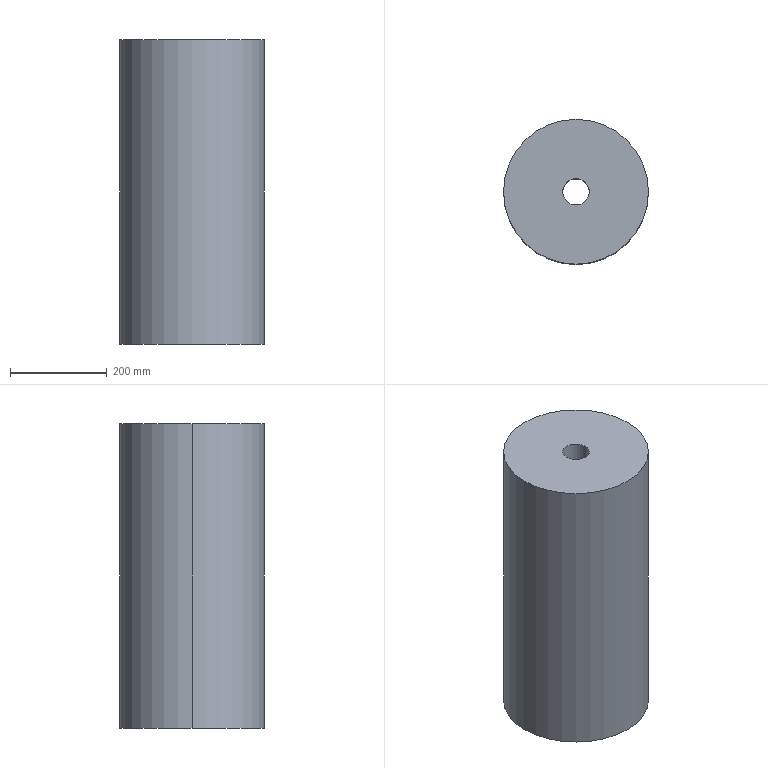Part | STEP file | Coil stock | 1 solid | 6 faces | box 300 x 300 x 630 mm | volume 43035303 mm3 | cylinder 4 | plane 2 | commonest cylinder face diameters 55 x2 300 x2
STEP:
#1=CARTESIAN_POINT('',(0.,0.,0.));
#2=DIRECTION('',(0.,0.,1.));
#3=DIRECTION('',(1.,0.,0.));
#4=AXIS2_PLACEMENT_3D('',#1,#2,#3);
#5=CARTESIAN_POINT('',(150.,0.,0.));
#6=VERTEX_POINT('',#5);
#7=CARTESIAN_POINT('',(-150.,0.,0.));
#8=VERTEX_POINT('',#7);
#9=CARTESIAN_POINT('',(0.,0.,0.));
#10=DIRECTION('',(0.,0.,1.));
#11=DIRECTION('',(1.,0.,0.));
#12=AXIS2_PLACEMENT_3D('',#9,#10,#11);
#13=CIRCLE('',#12,150.);
#14=CARTESIAN_POINT('',(0.,0.,0.));
#15=DIRECTION('',(0.,0.,1.));
#16=DIRECTION('',(1.,0.,0.));
#17=AXIS2_PLACEMENT_3D('',#14,#15,#16);
#18=CYLINDRICAL_SURFACE('',#17,150.);
#19=CARTESIAN_POINT('',(0.,0.));
#20=DIRECTION('',(1.,0.));
#21=VECTOR('',#20,1.);
#22=LINE('',#19,#21);
#23=(GEOMETRIC_REPRESENTATION_CONTEXT(2)PARAMETRIC_REPRESENTATION_CONTEXT()REPRESENTATION_CONTEXT('',''));
#24=DEFINITIONAL_REPRESENTATION('',(#22),#23);
#25=PCURVE('',#18,#24);
#26=CARTESIAN_POINT('',(0.,0.,0.));
#27=DIRECTION('',(0.,0.,-1.));
#28=DIRECTION('',(-1.,0.,0.));
#29=AXIS2_PLACEMENT_3D('',#26,#27,#28);
#30=PLANE('',#29);
#31=CARTESIAN_POINT('',(-150.,0.));
#32=CARTESIAN_POINT('',(-150.,259.808));
#33=CARTESIAN_POINT('',(75.,129.904));
#34=CARTESIAN_POINT('',(300.,0.));
#35=CARTESIAN_POINT('',(75.,-129.904));
#36=CARTESIAN_POINT('',(-150.,-259.808));
#37=CARTESIAN_POINT('',(-150.,0.));
#38=(BOUNDED_CURVE()B_SPLINE_CURVE(2,(#31,#32,#33,#34,#35,#36,#37),.UNSPECIFIED.,.T.,.F.)B_SPLINE_CURVE_WITH_KNOTS((1,2,2,2,2,1),(-2.094,0.,2.094,4.189,6.283,8.378),.UNSPECIFIED.)CURVE()GEOMETRIC_REPRESENTATION_ITEM()RATIONAL_B_SPLINE_CURVE((1.,0.5,1.,0.5,1.,0.5,1.))REPRESENTATION_ITEM(''));
#39=(GEOMETRIC_REPRESENTATION_CONTEXT(2)PARAMETRIC_REPRESENTATION_CONTEXT()REPRESENTATION_CONTEXT('',''));
#40=DEFINITIONAL_REPRESENTATION('',(#38),#39);
#41=PCURVE('',#30,#40);
#42=SURFACE_CURVE('',#13,(#25,#41),.PCURVE_S1.);
#43=EDGE_CURVE('',#6,#8,#42,.T.);
#44=ORIENTED_EDGE('',*,*,#43,.T.);
#45=CARTESIAN_POINT('',(-150.,0.,630.));
#46=VERTEX_POINT('',#45);
#47=CARTESIAN_POINT('',(-150.,0.,0.));
#48=DIRECTION('',(0.,0.,1.));
#49=VECTOR('',#48,1.);
#50=LINE('',#47,#49);
#51=CARTESIAN_POINT('',(3.142,0.));
#52=DIRECTION('',(0.,1.));
#53=VECTOR('',#52,1.);
#54=LINE('',#51,#53);
#55=(GEOMETRIC_REPRESENTATION_CONTEXT(2)PARAMETRIC_REPRESENTATION_CONTEXT()REPRESENTATION_CONTEXT('',''));
#56=DEFINITIONAL_REPRESENTATION('',(#54),#55);
#57=PCURVE('',#18,#56);
#58=CARTESIAN_POINT('',(0.,0.,0.));
#59=DIRECTION('',(0.,0.,1.));
#60=DIRECTION('',(1.,0.,0.));
#61=AXIS2_PLACEMENT_3D('',#58,#59,#60);
#62=CYLINDRICAL_SURFACE('',#61,150.);
#63=CARTESIAN_POINT('',(3.142,0.));
#64=DIRECTION('',(0.,1.));
#65=VECTOR('',#64,1.);
#66=LINE('',#63,#65);
#67=(GEOMETRIC_REPRESENTATION_CONTEXT(2)PARAMETRIC_REPRESENTATION_CONTEXT()REPRESENTATION_CONTEXT('',''));
#68=DEFINITIONAL_REPRESENTATION('',(#66),#67);
#69=PCURVE('',#62,#68);
#70=SURFACE_CURVE('',#50,(#57,#69),.PCURVE_S1.);
#71=EDGE_CURVE('',#8,#46,#70,.T.);
#72=ORIENTED_EDGE('',*,*,#71,.T.);
#73=CARTESIAN_POINT('',(150.,0.,630.));
#74=VERTEX_POINT('',#73);
#75=CARTESIAN_POINT('',(0.,0.,630.));
#76=DIRECTION('',(0.,0.,-1.));
#77=DIRECTION('',(1.,0.,0.));
#78=AXIS2_PLACEMENT_3D('',#75,#76,#77);
#79=CIRCLE('',#78,150.);
#80=CARTESIAN_POINT('',(6.283,630.));
#81=DIRECTION('',(-1.,0.));
#82=VECTOR('',#81,1.);
#83=LINE('',#80,#82);
#84=(GEOMETRIC_REPRESENTATION_CONTEXT(2)PARAMETRIC_REPRESENTATION_CONTEXT()REPRESENTATION_CONTEXT('',''));
#85=DEFINITIONAL_REPRESENTATION('',(#83),#84);
#86=PCURVE('',#18,#85);
#87=CARTESIAN_POINT('',(0.,0.,630.));
#88=DIRECTION('',(0.,0.,-1.));
#89=DIRECTION('',(-1.,0.,0.));
#90=AXIS2_PLACEMENT_3D('',#87,#88,#89);
#91=PLANE('',#90);
#92=CARTESIAN_POINT('',(0.,0.));
#93=DIRECTION('',(-1.,0.));
#94=AXIS2_PLACEMENT_2D('',#92,#93);
#95=CIRCLE('',#94,150.);
#96=(GEOMETRIC_REPRESENTATION_CONTEXT(2)PARAMETRIC_REPRESENTATION_CONTEXT()REPRESENTATION_CONTEXT('',''));
#97=DEFINITIONAL_REPRESENTATION('',(#95),#96);
#98=PCURVE('',#91,#97);
#99=SURFACE_CURVE('',#79,(#86,#98),.PCURVE_S1.);
#100=EDGE_CURVE('',#46,#74,#99,.T.);
#101=ORIENTED_EDGE('',*,*,#100,.T.);
#102=CARTESIAN_POINT('',(150.,0.,0.));
#103=DIRECTION('',(0.,0.,1.));
#104=VECTOR('',#103,1.);
#105=LINE('',#102,#104);
#106=CARTESIAN_POINT('',(0.,0.));
#107=DIRECTION('',(0.,1.));
#108=VECTOR('',#107,1.);
#109=LINE('',#106,#108);
#110=(GEOMETRIC_REPRESENTATION_CONTEXT(2)PARAMETRIC_REPRESENTATION_CONTEXT()REPRESENTATION_CONTEXT('',''));
#111=DEFINITIONAL_REPRESENTATION('',(#109),#110);
#112=PCURVE('',#18,#111);
#113=CARTESIAN_POINT('',(6.283,0.));
#114=DIRECTION('',(0.,1.));
#115=VECTOR('',#114,1.);
#116=LINE('',#113,#115);
#117=(GEOMETRIC_REPRESENTATION_CONTEXT(2)PARAMETRIC_REPRESENTATION_CONTEXT()REPRESENTATION_CONTEXT('',''));
#118=DEFINITIONAL_REPRESENTATION('',(#116),#117);
#119=PCURVE('',#62,#118);
#120=SURFACE_CURVE('',#105,(#112,#119),.PCURVE_S1.);
#121=EDGE_CURVE('',#6,#74,#120,.T.);
#122=ORIENTED_EDGE('',*,*,#121,.F.);
#123=EDGE_LOOP('',(#44,#72,#101,#122));
#124=FACE_BOUND('',#123,.T.);
#125=ADVANCED_FACE('',(#124),#18,.T.);
#126=CARTESIAN_POINT('',(27.5,0.,0.));
#127=VERTEX_POINT('',#126);
#128=CARTESIAN_POINT('',(27.5,0.,630.));
#129=VERTEX_POINT('',#128);
#130=CARTESIAN_POINT('',(27.5,0.,0.));
#131=DIRECTION('',(0.,0.,1.));
#132=VECTOR('',#131,1.);
#133=LINE('',#130,#132);
#134=CARTESIAN_POINT('',(0.,0.,0.));
#135=DIRECTION('',(0.,0.,1.));
#136=DIRECTION('',(1.,0.,0.));
#137=AXIS2_PLACEMENT_3D('',#134,#135,#136);
#138=CYLINDRICAL_SURFACE('',#137,27.5);
#139=CARTESIAN_POINT('',(6.283,0.));
#140=DIRECTION('',(0.,1.));
#141=VECTOR('',#140,1.);
#142=LINE('',#139,#141);
#143=(GEOMETRIC_REPRESENTATION_CONTEXT(2)PARAMETRIC_REPRESENTATION_CONTEXT()REPRESENTATION_CONTEXT('',''));
#144=DEFINITIONAL_REPRESENTATION('',(#142),#143);
#145=PCURVE('',#138,#144);
#146=CARTESIAN_POINT('',(0.,0.,0.));
#147=DIRECTION('',(0.,0.,1.));
#148=DIRECTION('',(1.,0.,0.));
#149=AXIS2_PLACEMENT_3D('',#146,#147,#148);
#150=CYLINDRICAL_SURFACE('',#149,27.5);
#151=CARTESIAN_POINT('',(0.,0.));
#152=DIRECTION('',(0.,1.));
#153=VECTOR('',#152,1.);
#154=LINE('',#151,#153);
#155=(GEOMETRIC_REPRESENTATION_CONTEXT(2)PARAMETRIC_REPRESENTATION_CONTEXT()REPRESENTATION_CONTEXT('',''));
#156=DEFINITIONAL_REPRESENTATION('',(#154),#155);
#157=PCURVE('',#150,#156);
#158=SURFACE_CURVE('',#133,(#145,#157),.PCURVE_S1.);
#159=EDGE_CURVE('',#127,#129,#158,.T.);
#160=ORIENTED_EDGE('',*,*,#159,.T.);
#161=CARTESIAN_POINT('',(-27.5,0.,630.));
#162=VERTEX_POINT('',#161);
#163=CARTESIAN_POINT('',(0.,0.,630.));
#164=DIRECTION('',(0.,0.,1.));
#165=DIRECTION('',(1.,0.,0.));
#166=AXIS2_PLACEMENT_3D('',#163,#164,#165);
#167=CIRCLE('',#166,27.5);
#168=CARTESIAN_POINT('',(0.,630.));
#169=DIRECTION('',(1.,0.));
#170=VECTOR('',#169,1.);
#171=LINE('',#168,#170);
#172=(GEOMETRIC_REPRESENTATION_CONTEXT(2)PARAMETRIC_REPRESENTATION_CONTEXT()REPRESENTATION_CONTEXT('',''));
#173=DEFINITIONAL_REPRESENTATION('',(#171),#172);
#174=PCURVE('',#138,#173);
#175=CARTESIAN_POINT('',(-27.5,0.));
#176=CARTESIAN_POINT('',(-27.5,47.631));
#177=CARTESIAN_POINT('',(13.75,23.816));
#178=CARTESIAN_POINT('',(55.,0.));
#179=CARTESIAN_POINT('',(13.75,-23.816));
#180=CARTESIAN_POINT('',(-27.5,-47.631));
#181=CARTESIAN_POINT('',(-27.5,0.));
#182=(BOUNDED_CURVE()B_SPLINE_CURVE(2,(#175,#176,#177,#178,#179,#180,#181),.UNSPECIFIED.,.T.,.F.)B_SPLINE_CURVE_WITH_KNOTS((1,2,2,2,2,1),(-2.094,0.,2.094,4.189,6.283,8.378),.UNSPECIFIED.)CURVE()GEOMETRIC_REPRESENTATION_ITEM()RATIONAL_B_SPLINE_CURVE((1.,0.5,1.,0.5,1.,0.5,1.))REPRESENTATION_ITEM(''));
#183=(GEOMETRIC_REPRESENTATION_CONTEXT(2)PARAMETRIC_REPRESENTATION_CONTEXT()REPRESENTATION_CONTEXT('',''));
#184=DEFINITIONAL_REPRESENTATION('',(#182),#183);
#185=PCURVE('',#91,#184);
#186=SURFACE_CURVE('',#167,(#174,#185),.PCURVE_S1.);
#187=EDGE_CURVE('',#162,#129,#186,.T.);
#188=ORIENTED_EDGE('',*,*,#187,.F.);
#189=CARTESIAN_POINT('',(-27.5,0.,0.));
#190=VERTEX_POINT('',#189);
#191=CARTESIAN_POINT('',(-27.5,0.,0.));
#192=DIRECTION('',(0.,0.,1.));
#193=VECTOR('',#192,1.);
#194=LINE('',#191,#193);
#195=CARTESIAN_POINT('',(3.142,0.));
#196=DIRECTION('',(0.,1.));
#197=VECTOR('',#196,1.);
#198=LINE('',#195,#197);
#199=(GEOMETRIC_REPRESENTATION_CONTEXT(2)PARAMETRIC_REPRESENTATION_CONTEXT()REPRESENTATION_CONTEXT('',''));
#200=DEFINITIONAL_REPRESENTATION('',(#198),#199);
#201=PCURVE('',#138,#200);
#202=CARTESIAN_POINT('',(3.142,0.));
#203=DIRECTION('',(0.,1.));
#204=VECTOR('',#203,1.);
#205=LINE('',#202,#204);
#206=(GEOMETRIC_REPRESENTATION_CONTEXT(2)PARAMETRIC_REPRESENTATION_CONTEXT()REPRESENTATION_CONTEXT('',''));
#207=DEFINITIONAL_REPRESENTATION('',(#205),#206);
#208=PCURVE('',#150,#207);
#209=SURFACE_CURVE('',#194,(#201,#208),.PCURVE_S1.);
#210=EDGE_CURVE('',#190,#162,#209,.T.);
#211=ORIENTED_EDGE('',*,*,#210,.F.);
#212=CARTESIAN_POINT('',(0.,0.,0.));
#213=DIRECTION('',(0.,0.,1.));
#214=DIRECTION('',(1.,0.,0.));
#215=AXIS2_PLACEMENT_3D('',#212,#213,#214);
#216=CIRCLE('',#215,27.5);
#217=CARTESIAN_POINT('',(0.,0.));
#218=DIRECTION('',(1.,0.));
#219=VECTOR('',#218,1.);
#220=LINE('',#217,#219);
#221=(GEOMETRIC_REPRESENTATION_CONTEXT(2)PARAMETRIC_REPRESENTATION_CONTEXT()REPRESENTATION_CONTEXT('',''));
#222=DEFINITIONAL_REPRESENTATION('',(#220),#221);
#223=PCURVE('',#138,#222);
#224=CARTESIAN_POINT('',(-27.5,0.));
#225=CARTESIAN_POINT('',(-27.5,47.631));
#226=CARTESIAN_POINT('',(13.75,23.816));
#227=CARTESIAN_POINT('',(55.,0.));
#228=CARTESIAN_POINT('',(13.75,-23.816));
#229=CARTESIAN_POINT('',(-27.5,-47.631));
#230=CARTESIAN_POINT('',(-27.5,0.));
#231=(BOUNDED_CURVE()B_SPLINE_CURVE(2,(#224,#225,#226,#227,#228,#229,#230),.UNSPECIFIED.,.T.,.F.)B_SPLINE_CURVE_WITH_KNOTS((1,2,2,2,2,1),(-2.094,0.,2.094,4.189,6.283,8.378),.UNSPECIFIED.)CURVE()GEOMETRIC_REPRESENTATION_ITEM()RATIONAL_B_SPLINE_CURVE((1.,0.5,1.,0.5,1.,0.5,1.))REPRESENTATION_ITEM(''));
#232=(GEOMETRIC_REPRESENTATION_CONTEXT(2)PARAMETRIC_REPRESENTATION_CONTEXT()REPRESENTATION_CONTEXT('',''));
#233=DEFINITIONAL_REPRESENTATION('',(#231),#232);
#234=PCURVE('',#30,#233);
#235=SURFACE_CURVE('',#216,(#223,#234),.PCURVE_S1.);
#236=EDGE_CURVE('',#190,#127,#235,.T.);
#237=ORIENTED_EDGE('',*,*,#236,.T.);
#238=EDGE_LOOP('',(#160,#188,#211,#237));
#239=FACE_BOUND('',#238,.F.);
#240=ADVANCED_FACE('',(#239),#138,.F.);
#241=ORIENTED_EDGE('',*,*,#71,.F.);
#242=CARTESIAN_POINT('',(0.,0.,0.));
#243=DIRECTION('',(0.,0.,1.));
#244=DIRECTION('',(1.,0.,0.));
#245=AXIS2_PLACEMENT_3D('',#242,#243,#244);
#246=CIRCLE('',#245,150.);
#247=CARTESIAN_POINT('',(0.,0.));
#248=DIRECTION('',(1.,0.));
#249=VECTOR('',#248,1.);
#250=LINE('',#247,#249);
#251=(GEOMETRIC_REPRESENTATION_CONTEXT(2)PARAMETRIC_REPRESENTATION_CONTEXT()REPRESENTATION_CONTEXT('',''));
#252=DEFINITIONAL_REPRESENTATION('',(#250),#251);
#253=PCURVE('',#62,#252);
#254=CARTESIAN_POINT('',(-150.,0.));
#255=CARTESIAN_POINT('',(-150.,259.808));
#256=CARTESIAN_POINT('',(75.,129.904));
#257=CARTESIAN_POINT('',(300.,0.));
#258=CARTESIAN_POINT('',(75.,-129.904));
#259=CARTESIAN_POINT('',(-150.,-259.808));
#260=CARTESIAN_POINT('',(-150.,0.));
#261=(BOUNDED_CURVE()B_SPLINE_CURVE(2,(#254,#255,#256,#257,#258,#259,#260),.UNSPECIFIED.,.T.,.F.)B_SPLINE_CURVE_WITH_KNOTS((1,2,2,2,2,1),(-2.094,0.,2.094,4.189,6.283,8.378),.UNSPECIFIED.)CURVE()GEOMETRIC_REPRESENTATION_ITEM()RATIONAL_B_SPLINE_CURVE((1.,0.5,1.,0.5,1.,0.5,1.))REPRESENTATION_ITEM(''));
#262=(GEOMETRIC_REPRESENTATION_CONTEXT(2)PARAMETRIC_REPRESENTATION_CONTEXT()REPRESENTATION_CONTEXT('',''));
#263=DEFINITIONAL_REPRESENTATION('',(#261),#262);
#264=PCURVE('',#30,#263);
#265=SURFACE_CURVE('',#246,(#253,#264),.PCURVE_S1.);
#266=EDGE_CURVE('',#8,#6,#265,.T.);
#267=ORIENTED_EDGE('',*,*,#266,.T.);
#268=ORIENTED_EDGE('',*,*,#121,.T.);
#269=CARTESIAN_POINT('',(0.,0.,630.));
#270=DIRECTION('',(0.,0.,-1.));
#271=DIRECTION('',(1.,0.,0.));
#272=AXIS2_PLACEMENT_3D('',#269,#270,#271);
#273=CIRCLE('',#272,150.);
#274=CARTESIAN_POINT('',(6.283,630.));
#275=DIRECTION('',(-1.,0.));
#276=VECTOR('',#275,1.);
#277=LINE('',#274,#276);
#278=(GEOMETRIC_REPRESENTATION_CONTEXT(2)PARAMETRIC_REPRESENTATION_CONTEXT()REPRESENTATION_CONTEXT('',''));
#279=DEFINITIONAL_REPRESENTATION('',(#277),#278);
#280=PCURVE('',#62,#279);
#281=CARTESIAN_POINT('',(0.,0.));
#282=DIRECTION('',(-1.,0.));
#283=AXIS2_PLACEMENT_2D('',#281,#282);
#284=CIRCLE('',#283,150.);
#285=(GEOMETRIC_REPRESENTATION_CONTEXT(2)PARAMETRIC_REPRESENTATION_CONTEXT()REPRESENTATION_CONTEXT('',''));
#286=DEFINITIONAL_REPRESENTATION('',(#284),#285);
#287=PCURVE('',#91,#286);
#288=SURFACE_CURVE('',#273,(#280,#287),.PCURVE_S1.);
#289=EDGE_CURVE('',#74,#46,#288,.T.);
#290=ORIENTED_EDGE('',*,*,#289,.T.);
#291=EDGE_LOOP('',(#241,#267,#268,#290));
#292=FACE_BOUND('',#291,.T.);
#293=ADVANCED_FACE('',(#292),#62,.T.);
#294=CARTESIAN_POINT('',(0.,0.,0.));
#295=DIRECTION('',(0.,0.,1.));
#296=DIRECTION('',(1.,0.,0.));
#297=AXIS2_PLACEMENT_3D('',#294,#295,#296);
#298=CIRCLE('',#297,27.5);
#299=CARTESIAN_POINT('',(-27.5,0.));
#300=CARTESIAN_POINT('',(-27.5,47.631));
#301=CARTESIAN_POINT('',(13.75,23.816));
#302=CARTESIAN_POINT('',(55.,0.));
#303=CARTESIAN_POINT('',(13.75,-23.816));
#304=CARTESIAN_POINT('',(-27.5,-47.631));
#305=CARTESIAN_POINT('',(-27.5,0.));
#306=(BOUNDED_CURVE()B_SPLINE_CURVE(2,(#299,#300,#301,#302,#303,#304,#305),.UNSPECIFIED.,.T.,.F.)B_SPLINE_CURVE_WITH_KNOTS((1,2,2,2,2,1),(-2.094,0.,2.094,4.189,6.283,8.378),.UNSPECIFIED.)CURVE()GEOMETRIC_REPRESENTATION_ITEM()RATIONAL_B_SPLINE_CURVE((1.,0.5,1.,0.5,1.,0.5,1.))REPRESENTATION_ITEM(''));
#307=(GEOMETRIC_REPRESENTATION_CONTEXT(2)PARAMETRIC_REPRESENTATION_CONTEXT()REPRESENTATION_CONTEXT('',''));
#308=DEFINITIONAL_REPRESENTATION('',(#306),#307);
#309=PCURVE('',#30,#308);
#310=CARTESIAN_POINT('',(0.,0.));
#311=DIRECTION('',(1.,0.));
#312=VECTOR('',#311,1.);
#313=LINE('',#310,#312);
#314=(GEOMETRIC_REPRESENTATION_CONTEXT(2)PARAMETRIC_REPRESENTATION_CONTEXT()REPRESENTATION_CONTEXT('',''));
#315=DEFINITIONAL_REPRESENTATION('',(#313),#314);
#316=PCURVE('',#150,#315);
#317=SURFACE_CURVE('',#298,(#309,#316),.PCURVE_S1.);
#318=EDGE_CURVE('',#127,#190,#317,.T.);
#319=ORIENTED_EDGE('',*,*,#318,.T.);
#320=ORIENTED_EDGE('',*,*,#236,.T.);
#321=EDGE_LOOP('',(#319,#320));
#322=FACE_BOUND('',#321,.T.);
#323=ORIENTED_EDGE('',*,*,#43,.F.);
#324=ORIENTED_EDGE('',*,*,#266,.F.);
#325=EDGE_LOOP('',(#323,#324));
#326=FACE_BOUND('',#325,.T.);
#327=ADVANCED_FACE('',(#322,#326),#30,.T.);
#328=CARTESIAN_POINT('',(0.,0.,630.));
#329=DIRECTION('',(0.,0.,1.));
#330=DIRECTION('',(1.,0.,0.));
#331=AXIS2_PLACEMENT_3D('',#328,#329,#330);
#332=CIRCLE('',#331,27.5);
#333=CARTESIAN_POINT('',(-27.5,0.));
#334=CARTESIAN_POINT('',(-27.5,47.631));
#335=CARTESIAN_POINT('',(13.75,23.816));
#336=CARTESIAN_POINT('',(55.,0.));
#337=CARTESIAN_POINT('',(13.75,-23.816));
#338=CARTESIAN_POINT('',(-27.5,-47.631));
#339=CARTESIAN_POINT('',(-27.5,0.));
#340=(BOUNDED_CURVE()B_SPLINE_CURVE(2,(#333,#334,#335,#336,#337,#338,#339),.UNSPECIFIED.,.T.,.F.)B_SPLINE_CURVE_WITH_KNOTS((1,2,2,2,2,1),(-2.094,0.,2.094,4.189,6.283,8.378),.UNSPECIFIED.)CURVE()GEOMETRIC_REPRESENTATION_ITEM()RATIONAL_B_SPLINE_CURVE((1.,0.5,1.,0.5,1.,0.5,1.))REPRESENTATION_ITEM(''));
#341=(GEOMETRIC_REPRESENTATION_CONTEXT(2)PARAMETRIC_REPRESENTATION_CONTEXT()REPRESENTATION_CONTEXT('',''));
#342=DEFINITIONAL_REPRESENTATION('',(#340),#341);
#343=PCURVE('',#91,#342);
#344=CARTESIAN_POINT('',(0.,630.));
#345=DIRECTION('',(1.,0.));
#346=VECTOR('',#345,1.);
#347=LINE('',#344,#346);
#348=(GEOMETRIC_REPRESENTATION_CONTEXT(2)PARAMETRIC_REPRESENTATION_CONTEXT()REPRESENTATION_CONTEXT('',''));
#349=DEFINITIONAL_REPRESENTATION('',(#347),#348);
#350=PCURVE('',#150,#349);
#351=SURFACE_CURVE('',#332,(#343,#350),.PCURVE_S1.);
#352=EDGE_CURVE('',#129,#162,#351,.T.);
#353=ORIENTED_EDGE('',*,*,#352,.F.);
#354=ORIENTED_EDGE('',*,*,#187,.F.);
#355=EDGE_LOOP('',(#353,#354));
#356=FACE_BOUND('',#355,.T.);
#357=ORIENTED_EDGE('',*,*,#289,.F.);
#358=ORIENTED_EDGE('',*,*,#100,.F.);
#359=EDGE_LOOP('',(#357,#358));
#360=FACE_BOUND('',#359,.T.);
#361=ADVANCED_FACE('',(#356,#360),#91,.F.);
#362=ORIENTED_EDGE('',*,*,#352,.F.);
#363=ORIENTED_EDGE('',*,*,#159,.F.);
#364=ORIENTED_EDGE('',*,*,#318,.T.);
#365=ORIENTED_EDGE('',*,*,#210,.T.);
#366=EDGE_LOOP('',(#362,#363,#364,#365));
#367=FACE_BOUND('',#366,.F.);
#368=ADVANCED_FACE('',(#367),#150,.F.);
#369=CLOSED_SHELL('',(#125,#240,#293,#327,#361,#368));
#370=MANIFOLD_SOLID_BREP('',#369);
#371=(LENGTH_UNIT()NAMED_UNIT(*)SI_UNIT(.MILLI.,.METRE.));
#372=UNCERTAINTY_MEASURE_WITH_UNIT(LENGTH_MEASURE(0.0000001),#371,'','');
#373=(NAMED_UNIT(*)PLANE_ANGLE_UNIT()SI_UNIT($,.RADIAN.));
#374=(NAMED_UNIT(*)SI_UNIT($,.STERADIAN.)SOLID_ANGLE_UNIT());
#375=(GEOMETRIC_REPRESENTATION_CONTEXT(3)GLOBAL_UNCERTAINTY_ASSIGNED_CONTEXT((#372))GLOBAL_UNIT_ASSIGNED_CONTEXT((#371,#373,#374))REPRESENTATION_CONTEXT('',''));
#376=ADVANCED_BREP_SHAPE_REPRESENTATION('',(#4,#370),#375);